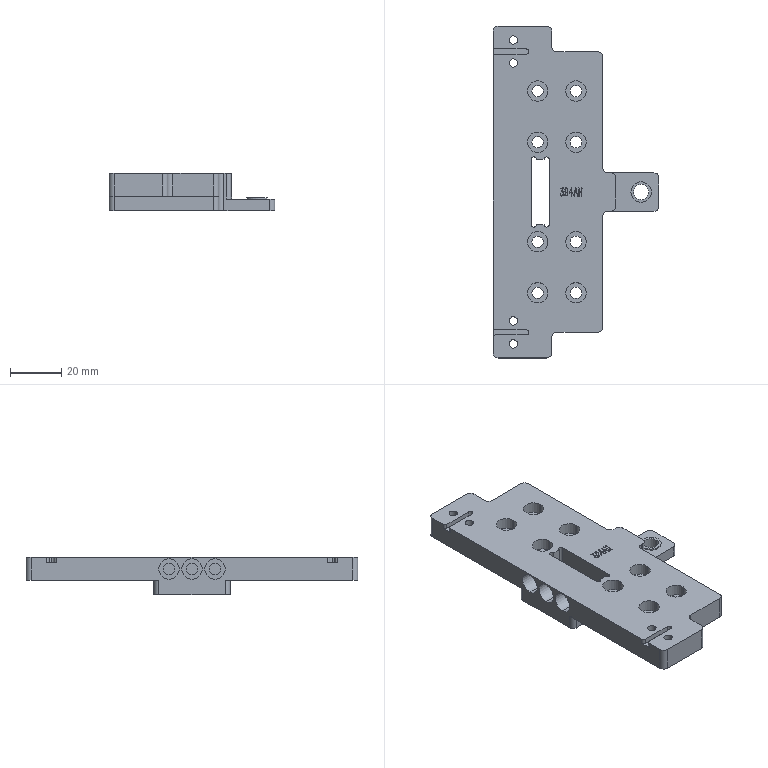NC program | NX | posted with a generic post | part box 65 x 130 x 14.5 mm
Lines 108 to 1017 of 11202:
(ADAPTIVE_MILLING , TOOL : D10)
N178 T15 M6
N180 G54
N182 G17 G0 G90 X0.062 Y-45.209 B0. C0. S9500 M3
N184 G43 Z30. H15
N186 Z-11.5
N188 G94 G1 Z-14.5 F1000.
N190 X0.341 Y-44.428 F3000.
N192 X0.597 Y-43.64
N194 G3 X0.062 Y-42.562 R1.017
N196 X-3.002 Y-41.801 R8.28
N198 X-12.869 Y-41.519 R111.643
N200 G1 X-15.119 Y-41.514
N202 X-18.994 Y-41.511
N204 X-32.619 Y-41.51
N206 X-66.869
N208 X-66.994 Y-41.509
N210 X-67.119 Y-41.508
N212 G2 X-71.4 Y-39.014 R5.714
N214 X-73.465 Y-33.574 R12.314
N216 X-73.953 Y-25.471 R57.528
N218 G1 X-73.962 Y-24.596
N220 X-73.971 Y-23.346
N222 X-73.978 Y-21.721
N224 X-73.983 Y-19.596
N226 X-73.987 Y-16.096
N228 X-73.988 Y-6.096
N230 Y34.529
N232 X-73.986 Y34.654
N234 X-73.979 Y34.779
N236 X-73.969 Y34.903
N238 G2 X-71.265 Y39.069 R5.937
N240 X-65.65 Y41.03 R13.149
N242 X-57.042 Y41.463 R69.652
N244 G1 X-55.792 Y41.472
N246 X-54.167 Y41.479
N248 X-51.917 Y41.484
N250 X-48.167 Y41.487
N252 X-36.542 Y41.488
N254 X66.958
N256 G2 X71.225 Y39.219 R5.583
N258 X73.439 Y33.711 R11.905
N260 X73.949 Y25.735 R53.792
N262 G1 X73.959 Y24.86
N264 X73.969 Y23.61
N266 X73.976 Y22.235
N268 X73.982 Y20.36
N270 X73.986 Y17.485
N272 X73.988 Y11.36
N274 Y-34.515
N276 X73.986 Y-34.639
N278 X73.98 Y-34.764
N280 X73.97 Y-34.889
N282 G2 X71.274 Y-39.06 R5.924
N284 X65.538 Y-41.044 R13.207
N286 X56.429 Y-41.467 R75.516
N288 G1 X55.054 Y-41.475
N290 X53.429 Y-41.481
N292 X50.929 Y-41.485
N294 X46.304 Y-41.488
N296 X7.804
N298 X3.804
N300 G2 X-1.419 Y-40.99 R59.156
N302 G3 X-13.656 Y-40.537 R126.191
N304 G1 X-15.531 Y-40.53
N306 X-18.031 Y-40.525
N308 X-22.031 Y-40.522
N310 X-33.531 Y-40.521
N312 X-63.906
N314 X-64.031 Y-40.519
N316 G2 X-70.336 Y-36.815 R7.665
N318 X-72.471 Y-30.468 R15.611
N320 X-72.94 Y-21.611 R73.657
N322 G1 X-72.952 Y-20.361
N324 X-72.961 Y-18.986
N326 X-72.968 Y-17.236
N328 X-72.973 Y-14.736
N330 X-72.976 Y-10.736
N332 X-72.977 Y2.389
N334 Y31.389
N336 X-72.975 Y31.639
N338 X-72.97 Y31.764
N340 X-72.964 Y31.889
N342 G2 X-69.191 Y37.896 R7.687
N344 X-62.704 Y40.003 R15.904
N346 X-53.345 Y40.449 R81.636
N348 G1 X-52.095 Y40.458
N350 X-50.345 Y40.466
N352 X-48.345 Y40.472
N354 X-45.22 Y40.475
N356 X-38.595 Y40.477
N358 X63.905 Y40.478
N360 X64.03 Y40.477
N362 X64.155 Y40.473
N364 X64.28 Y40.469
N366 X64.405 Y40.462
N368 X64.529 Y40.453
N370 G2 X70.47 Y36.567 R7.761
N372 X72.519 Y30.059 R16.204
N374 X72.954 Y20.075 R89.33
N376 G1 X72.963 Y18.575
N378 X72.969 Y16.7
N380 X72.974 Y13.95
N382 X72.977 Y9.075
N384 Y-23.675
N386 Y-31.425
N388 G2 X69.367 Y-37.779 R7.596
N390 X63.158 Y-39.93 R15.098
N392 X53.804 Y-40.444 R72.251
N394 G1 X52.679 Y-40.454
N396 X51.429 Y-40.461
N398 X49.679 Y-40.468
N400 X47.304 Y-40.473
N402 X43.304 Y-40.476
N404 X31.429 Y-40.478
N406 X6.179
N408 X5.804 Y-40.475
N410 X5.679 Y-40.474
N412 X5.304 Y-40.466
N414 X5.054 Y-40.459
N416 G2 X-3.547 Y-39.831 R349.282
N418 G3 X-18.792 Y-39.538 R283.39
N420 G1 X-22.167 Y-39.534
N422 X-28.417 Y-39.532
N424 X-60.917 Y-39.531
N426 X-61.292 Y-39.53
N428 X-61.417 Y-39.528
N430 X-61.792 Y-39.518
N432 G2 X-69.405 Y-34.81 R8.956
N434 X-71.463 Y-28.038 R17.941
N436 X-71.938 Y-17.68 R90.973
N438 G1 X-71.948 Y-16.305
N440 X-71.955 Y-14.555
N442 X-71.961 Y-12.18
N444 X-71.965 Y-8.555
N446 X-71.966 Y-0.555
N448 X-71.967 Y28.82
N450 G2 X-67.242 Y36.921 R8.928
N452 X-60.467 Y38.972 R18.132
N454 X-51.109 Y39.43 R84.153
N456 G1 X-49.859 Y39.441
N458 X-48.359 Y39.45
N460 X-46.609 Y39.457
N462 X-44.109 Y39.462
N464 X-40.109 Y39.465
N466 X-28.984 Y39.467
N468 X61.266
N470 X61.516 Y39.465
N472 X61.641 Y39.462
N474 X61.766 Y39.459
N476 X61.891 Y39.454
N478 X62.141 Y39.443
N480 G2 X69.455 Y34.676 R8.935
N482 X71.494 Y27.768 R18.331
N484 X71.945 Y16.658 R104.558
N486 G1 X71.953 Y15.033
N488 X71.959 Y13.033
N490 X71.964 Y9.908
N492 X71.966 Y4.033
N494 X71.967 Y-28.717
N496 X71.963 Y-29.092
N498 G2 X67.433 Y-36.803 R8.865
N500 X60.438 Y-38.967 R17.814
N502 X50.08 Y-39.438 R93.921
N504 G1 X48.705 Y-39.448
N506 X46.955 Y-39.455
N508 X44.58 Y-39.461
N510 X40.955 Y-39.465
N512 X33.205 Y-39.467
N514 X7.955
N516 G2 X-1.281 Y-38.989 R139.831
N518 G3 X-19.272 Y-38.552 R278.015
N520 G1 X-22.147 Y-38.547
N522 X-26.772 Y-38.544
N524 X-38.772 Y-38.542
N526 X-57.897
N528 X-58.647 Y-38.538
N530 X-59.147 Y-38.532
N532 G2 X-64.007 Y-37.537 R11.586
N534 G1 X-64.532 Y-37.477
N536 X-64.647 Y-37.451
N538 G2 X-68.548 Y-35. R7.671
N540 X-69.977 Y-32.032 R8.027
N542 X-70.926 Y-15.936 R118.648
N544 G1 X-70.936 Y-14.436
N546 X-70.943 Y-12.561
N548 X-70.949 Y-10.061
N550 X-70.953 Y-6.436
N552 X-70.955 Y0.939
N554 X-70.956 Y26.439
N556 G2 X-69.229 Y32.715 R10.337
N558 X-63.063 Y36.975 R11.915
N560 X-55.185 Y38.236 R31.194
N562 X-39.314 Y38.453 R340.669
N564 G1 X-33.189 Y38.456
N566 X58.936
N568 X59.186 Y38.455
N570 X59.436 Y38.451
N572 X59.561 Y38.448
N574 X59.811 Y38.44
N576 G2 X68.387 Y33.084 R9.805
N578 X70.469 Y25.797 R19.905
N580 X70.928 Y14.937 R106.106
N582 G1 X70.938 Y13.437
N584 X70.945 Y11.562
N586 X70.95 Y9.062
N588 X70.954 Y5.062
N590 X70.956 Y-4.313
N592 Y-26.438
N594 G2 X70.056 Y-31.334 R11.594
N596 G1 X69.977 Y-32.032
N598 X69.951 Y-32.147
N600 G2 X67.5 Y-36.048 R7.671
N602 X64.532 Y-37.477 R8.027
N604 X48.56 Y-38.425 R119.399
N606 G1 X47.06 Y-38.435
N608 X45.185 Y-38.443
N610 X42.811 Y-38.449
N612 X39.311 Y-38.453
N614 X32.561 Y-38.456
N616 X9.311
N618 G2 X-1.302 Y-37.985 R191.273
N620 G3 X-10.298 Y-37.65 R326.947
N622 G1 X-62.97
N624 X-63.03 Y-37.647
N626 X-64.023 Y-37.535
N628 X-64.336 Y-37.5
N630 X-64.647 Y-37.451
N632 G2 X-68.548 Y-35. R7.671
N634 X-69.977 Y-32.032 R8.027
N636 G1 X-70.147 Y-30.53
N638 X-70.15 Y-30.47
N640 Y-11.53
N642 G3 X-69.97 Y-0.473 R205.799
N644 G1 X-69.967 Y3.777
N646 Y23.402
N648 X-69.962 Y24.152
N650 X-69.957 Y24.652
N652 X-69.95 Y25.026
N654 X-69.943 Y25.276
N656 G2 X-64.046 Y34.868 R10.551
N658 X-56.746 Y36.921 R21.229
N660 X-46.138 Y37.409 R100.126
N662 G1 X-44.763 Y37.42
N664 X-43.138 Y37.429
N666 X-41.013 Y37.436
N668 X-38.138 Y37.441
N670 X-33.263 Y37.444
N672 X-17.013 Y37.445
N674 X-7.263
N676 X-7.138 Y37.453
N678 X-7.032 Y37.477
N680 X-5.53 Y37.647
N682 X-5.47 Y37.65
N684 X5.47
N686 G3 X17.277 Y37.47 R222.549
N688 G1 X22.277 Y37.467
N690 X55.902
N692 X56.652 Y37.462
N694 X57.152 Y37.457
N696 X57.527 Y37.451
N698 X57.776 Y37.443
N700 G2 X67.481 Y31.321 R10.587
N702 X69.447 Y23.994 R21.803
N704 X69.916 Y12.759 R111.443
N706 G1 X69.926 Y11.259
N708 X69.933 Y9.384
N710 X69.939 Y6.884
N712 X69.943 Y3.134
N714 X69.945 Y-4.866
N716 Y-9.741
N718 X69.954 Y-9.865
N720 X69.977 Y-9.968
N722 X70.147 Y-11.47
N724 X70.15 Y-11.53
N726 Y-30.47
N728 X70.147 Y-30.53
N730 X70.049 Y-31.399
N732 G3 X71.963 Y-31.902 R1.
N734 G1 X72.643 Y-30.022 Z-14.4
N736 X73.171 Y-28.556
N738 X73.212 Y-28.389
N740 X73.231 Y-28.217
N742 Y16.158
N744 G3 X72.448 Y24.837 R48.938
N746 G1 X71.853 Y28.03
N748 G3 X69.966 Y33.165 R21.419
N750 X67.55 Y36.479 R15.331
N752 X64.589 Y38.702 R15.278
N754 X59.631 Y40.225 R13.173
N756 X53.401 Y40.489 R88.661
N758 G1 X8.712 Y40.829
N760 X8.525 Y40.808
N762 X8.342 Y40.761
N764 X6.542 Y40.062
N766 X5.834 Y39.793 Z-14.438
N768 X5.135 Y39.502 Z-14.476
N770 X4.945 Y39.353 Z-14.488
N772 X4.791 Y39.167 Z-14.5
N774 G3 X5.53 Y37.647 R1.002
N776 G2 X8.218 Y37.109 R8.94
N778 G3 X14.307 Y36.551 R31.104
N780 X27.432 Y36.478 R710.533
N782 G1 X47.432
N784 X52.932
N786 X54.057 Y36.471
N788 X55.057 Y36.463
N790 X55.432 Y36.457
N792 G2 X61.375 Y35.23 R13.199
N794 X66.904 Y28.858 R11.902
N796 X68.543 Y21.185 R26.67
N798 X68.914 Y9.445 R144.37
N800 G1 X68.922 Y7.445
N802 X68.928 Y4.82
N804 X68.932 Y0.945
N806 X68.934 Y-6.68
N808 X68.937 Y-7.18
N810 X68.938 Y-7.305
N812 G3 X69.41 Y-8.347 R2.177
N814 G1 X69.462 Y-8.454
N816 X69.951 Y-9.853
N818 X69.977 Y-9.968
N820 G3 X71.777 Y-10.311 R1.001
N822 X71.964 Y-9.624 Z-14.464 R1.251
N824 G1 X72.06 Y-8.351 Z-14.4
N826 X72.227 Y-6.071
N828 Y12.679
N830 G3 X71.467 Y22.621 R65.951
N832 G1 X70.865 Y26.447
N834 G3 X69.412 Y31.071 R19.913
N836 X65.701 Y35.996 R14.244
N838 X59.036 Y39.105 R12.236
N840 X54.69 Y39.47 R37.522
N842 G1 X10.919 Y40.427
N844 X10.704 Y40.404
N846 X10.496 Y40.343
N848 X8.72 Y39.566
N850 X8.114 Y39.306 Z-14.433
N852 X7.517 Y39.024 Z-14.466
N854 G3 X7.115 Y38.492 Z-14.5 R1.039
N856 X7.737 Y37.245 R1.005
N858 G2 X9.436 Y36.523 R12.4
N860 G3 X14.6 Y35.68 R18.818
N862 X26.722 Y35.493 R258.293
N864 G1 X30.722 Y35.49
N866 X42.597 Y35.488
N868 X49.847
N870 X50.347 Y35.486
N872 X53.222 Y35.465
N874 X53.597 Y35.461
N876 G2 X59.47 Y34.452 R15.167
N878 X65.585 Y28.143 R11.91
N880 X67.465 Y20.275 R25.475
N882 X67.904 Y7.162 R147.503
N884 G3 X67.964 Y-5.713 R786.636
N886 X68.622 Y-7.093 R1.753
N888 G1 X69.087 Y-7.833
N890 G3 X70.475 Y-8.142 R1.004
N892 X70.949 Y-7.235 Z-14.447 R1.113
N894 G1 X71.06 Y-6.308 Z-14.4
N896 X71.337 Y-3.936
N898 Y11.064
N900 G3 X70.515 Y20.996 R60.929
N902 G1 X69.954 Y24.279
N904 G3 X68.246 Y29.569 R23.438
N906 X66.391 Y32.578 R17.281
N908 G1 X65.44 Y33.814
N910 X64.452 Y35.023
N912 G3 X63.502 Y35.812 R4.158
N914 G1 X62.509 Y36.405
N916 X61.491 Y36.954
N918 G3 X58.259 Y37.964 R12.606
N920 X55.294 Y38.29 R21.54
N922 X44.055 Y38.612 R487.31
N924 G1 X12.656 Y39.094
N926 X10.323 Y38.822
N928 X9.663 Y38.748 Z-14.433
N930 X9.007 Y38.649 Z-14.466
N932 G3 X8.472 Y38.264 Z-14.5 R1.04
N934 X8.759 Y36.844 R1.004
N936 X13.595 Y35.011 R9.961
N938 X22.951 Y34.534 R74.786
N940 G1 X24.076 Y34.524
N942 X25.576 Y34.515
N944 X27.451 Y34.508
N946 X30.076 Y34.503
N948 X34.451 Y34.5
N950 X46.826 Y34.499
N952 G2 X54.323 Y34.341 R110.325
N954 X64.232 Y27.506 R11.875
N956 X66.331 Y19.826 R23.732
N958 X66.868 Y8.595 R103.424
N960 G3 X66.975 Y-4.279 R570.276
N962 X67.296 Y-5.729 R3.252
N964 G1 X67.371 Y-5.829
N966 X67.451 Y-5.913
N968 X67.5 Y-5.952
N970 X68.296 Y-6.748
N972 G3 X69.493 Y-6.912 R1.007
N974 X70.02 Y-6.026 Z-14.446 R1.11
N976 G1 X70.175 Y-5.114 Z-14.4
N978 X70.531 Y-3.018
N980 X70.546 Y-2.85
N982 X70.552 Y2.304
N984 X70.532 Y7.459
N986 G3 X69.662 Y18.337 R88.999
N988 G1 X68.944 Y23.283
N990 G3 X66.499 Y29.632 R17.756
N992 X63.652 Y33.467 R33.142
N994 X61.538 Y35.095 R8.254
N996 X57.53 Y36.767 R19.734
N998 X54.779 Y37.262 R17.832
N1000 G1 X53.381 Y37.384
N1002 X51.98 Y37.452
N1004 X13.805 Y38.372
N1006 X13.638 Y38.362
N1008 X11.517 Y38.056
N1010 X10.867 Y37.968 Z-14.433
N1012 X10.221 Y37.854 Z-14.466
N1014 G3 X9.688 Y37.442 Z-14.5 R1.039
N1016 X9.907 Y36.122 R1.005
N1018 X13.061 Y34.458 R6.193
N1020 X20.002 Y33.656 R34.038
N1022 X40.876 Y33.51 R729.268
N1024 G2 X52.374 Y33.382 R246.99
N1026 X60.504 Y30.01 R12.436
N1028 X64.46 Y22.881 R15.607
N1030 X65.685 Y13.857 R42.285
N1032 X65.927 Y-1.765 R504.611
N1034 G3 X66.356 Y-4.972 R10.178
N1036 X66.728 Y-5.451 R1.974
N1038 G1 X67.407 Y-5.878
N1040 X67.5 Y-5.952
N1042 G3 X68.593 Y-6.053 R1.01
N1044 X69.141 Y-5.185 Z-14.447 R1.112
N1046 G1 X69.324 Y-4.273 Z-14.4
N1048 X69.745 Y-2.154
N1050 X69.749 Y0.811
N1052 X69.736 Y3.777
N1054 G3 X69.239 Y11.04 R76.64
N1056 G1 X68.071 Y20.972
N1058 G3 X66.059 Y27.351 R18.53
N1060 X63.548 Y31.057 R19.959
N1062 G1 X62.05 Y32.782
N1064 G3 X59.881 Y34.33 R7.933
N1066 X55.808 Y35.836 R19.367
N1068 G1 X54.894 Y36.009
N1070 X53.972 Y36.128
N1072 G3 X46.502 Y36.661 R140.558
N1074 G1 X14.056 Y38.032
N1076 X11.925 Y37.669
N1078 X11.278 Y37.563 Z-14.433
N1080 X10.636 Y37.432 Z-14.466
N1082 G3 X10.114 Y37.004 Z-14.5 R1.038
N1084 X10.265 Y35.783 R1.007
N1086 X14.066 Y33.558 R6.919
N1088 X21.375 Y32.684 R35.467
N1090 X41.373 Y32.519 R649.43
N1092 G2 X51.245 Y32.361 R184.013
N1094 X59.453 Y28.85 R12.682
N1096 X63.438 Y21.594 R15.962
N1098 X64.678 Y12.194 R43.946
N1100 X64.939 Y-0.928 R757.799
N1102 G3 X65.511 Y-4.488 R10.583
N1104 X66.153 Y-5.09 R1.269
N1106 G1 X66.788 Y-5.489
N1108 G3 X67.857 Y-5.486 R1.011
N1110 X68.336 Y-4.695 Z-14.452 R1.141
N1112 G1 X68.584 Y-3.679 Z-14.4
N1114 X69.013 Y-1.919
N1116 X69.035 Y-1.756
N1118 X69.038 Y-1.592
N1120 X67.34 Y17.081
N1122 G3 X64.735 Y26.656 R28.478
N1124 G1 X64.115 Y27.973
N1126 X63.477 Y29.281
N1128 G3 X62.196 Y30.876 R6.306
N1130 X60.187 Y32.344 R13.52
N1132 G1 X58.031 Y33.605
N1134 G3 X54.422 Y34.899 R13.803
N1136 X51.465 Y35.296 R19.423
N1138 G1 X14.945 Y37.25
N1140 X14.691 Y37.231
N1142 X12.77 Y36.837
N1144 X12.117 Y36.708 Z-14.433
N1146 X11.469 Y36.556 Z-14.467
N1148 G3 X10.969 Y36.132 Z-14.5 R1.04
N1150 X11.048 Y35. R1.01
N1152 X13.483 Y33.144 R4.764
N1154 X19.71 Y31.891 R21.941
N1156 X33.328 Y31.544 R186.85
N1158 G2 X48.951 Y31.42 R720.332
N1160 X55.686 Y29.76 R15.123
N1162 X61.612 Y22.737 R13.595
N1164 X63.436 Y14.211 R30.177
N1166 X63.886 Y1.471 R195.494
N1168 G3 X64.399 Y-3.364 R20.481
N1170 X65.108 Y-4.659 R2.532
N1172 X66.031 Y-5.033 R5.554
N1174 X67.056 Y-4.808 R1.011
N1176 X67.355 Y-3.944 Z-14.453 R1.045
N1178 G1 X67.303 Y-2.893 Z-14.4
N1180 X67.196 Y-0.686
N1182 X67.199 Y3.062
N1184 X67.184 Y6.811
N1186 G3 X66.435 Y15.505 R66.209
N1188 G1 X65.834 Y19.331
N1190 G3 X63.076 Y26.434 R20.586
N1192 X61.18 Y29.178 R29.442
N1194 X57.298 Y32.365 R13.139
N1196 X52.012 Y34.101 R15.564
N1198 X48.287 Y34.439 R41.618
N1200 G1 X15.538 Y35.865
N1202 X13.33 Y36.102
N1204 X12.683 Y36.177 Z-14.433
N1206 X12.034 Y36.226 Z-14.465
N1208 G3 X11.409 Y35.949 Z-14.5 R1.038
N1210 X11.255 Y34.696 R1.007
N1212 X14.048 Y32.32 R5.139
N1214 X20.255 Y30.972 R21.659
N1216 X32.619 Y30.566 R150.127
N1218 G2 X47.618 Y30.419 R690.232
N1220 X54.482 Y28.755 R15.699
N1222 X60.481 Y21.791 R13.69
N1224 X62.393 Y13.16 R29.577
N1226 X62.87 Y2.422 R176.912
N1228 G3 X63.426 Y-2.661 R23.392
N1230 X64.234 Y-4.329 R3.629
N1232 X65.355 Y-4.797 R4.211
N1234 X66.415 Y-4.536 R1.01
N1236 X66.679 Y-3.704 Z-14.455 R1.051
N1238 G1 X66.626 Y-2.607 Z-14.4
N1240 X66.508 Y0.031
N1242 X66.442 Y2.67
N1244 G3 X65.978 Y8.887 R64.502
N1246 G1 X65.402 Y13.54
N1248 X64.804 Y18.19
N1250 G3 X62.487 Y24.6 R19.116
N1252 G1 X61.696 Y25.982
N1254 X60.89 Y27.356
N1256 G3 X59.53 Y28.885 R7.197
N1258 X56.138 Y31.324 R27.641
N1260 X52.511 Y32.731 R13.66
N1262 X49.438 Y33.215 R20.528
N1264 G1 X46.951 Y33.435
N1266 X44.46 Y33.608
N1268 X15.951 Y35.229
N1270 X13.737 Y35.466
N1272 X13.087 Y35.541 Z-14.433
N1274 X12.435 Y35.591 Z-14.466
N1276 G3 X11.814 Y35.32 Z-14.5 R1.038
N1278 X11.654 Y34.061 R1.007
N1280 X14.448 Y31.54 R5.23
N1282 X20.873 Y30.041 R21.18
N1284 X32.11 Y29.593 R127.475
N1286 G2 X46.483 Y29.411 R554.904
N1288 X53.452 Y27.662 R15.796
N1290 X59.479 Y20.559 R13.94
N1292 X61.341 Y12.295 R29.893
N1294 X61.894 Y2.187 R220.15
N1296 G3 X62.707 Y-2.855 R18.132
N1298 X63.641 Y-4.306 R3.138
N1300 X64.647 Y-4.549 R2.756
N1302 X65.59 Y-4.268 R1.014
N1304 X65.867 Y-3.371 Z-14.452 R1.133
N1306 G1 X65.85 Y-2.341 Z-14.4
N1308 X65.812 Y-0.202
N1310 X64.087 Y15.327
N1312 G3 X61.957 Y22.458 R21.485
N1314 G1 X60.835 Y24.684
N1316 G3 X58.138 Y28.033 R12.939
N1318 X54.034 Y30.807 R15.608
N1320 X50.469 Y31.857 R14.551
N1322 X45.526 Y32.513 R45.278
N1324 G1 X16.282 Y34.712
N1326 X14.136 Y34.817
N1328 X13.464 Y34.855 Z-14.434
N1330 X12.791 Y34.87 Z-14.467
N1332 G3 X12.211 Y34.595 Z-14.5 R1.041
N1334 X11.962 Y33.546 R1.01
N1336 X13.819 Y31.285 R3.896
N1338 X19.1 Y29.449 R14.901
N1340 X29.435 Y28.664 R69.044
N1342 G2 X45.183 Y28.418 R972.185
N1344 X52.059 Y26.78 R16.577
N1346 X58.367 Y19.61 R13.894
N1348 X60.368 Y10.615 R30.508
N1350 G1 X60.402 Y10.242
N1352 X60.434 Y9.868
N1354 X60.482 Y9.245
N1356 X60.518 Y8.746
N1358 X60.56 Y8.123
N1360 X60.598 Y7.499
N1362 X60.654 Y6.501
N1364 X60.734 Y5.003
N1366 X60.779 Y4.254
N1368 X60.834 Y3.381
N1370 X60.876 Y2.757
N1372 X60.916 Y2.259
N1374 X60.948 Y1.885
N1376 X60.983 Y1.512
N1378 G3 X62.053 Y-3.092 R13.998
N1380 X63.077 Y-4.314 R2.455
N1382 X64.047 Y-4.468 R6.205
N1384 X64.954 Y-4.08 R1.014
N1386 X65.162 Y-3.297 Z-14.459 R1.193
N1388 G1 X65.184 Y-2.125 Z-14.4
N1390 X65.207 Y-1.123
N1392 X65.211 Y-0.121
N1394 X64.443 Y5.951
N1396 G3 X63.256 Y12.842 R116.68
N1398 G1 X62.807 Y15.046
N1400 X62.342 Y17.248
N1402 G3 X59.441 Y23.963 R21.185
N1404 X57.732 Y26.421 R28.578
N1406 X55.48 Y28.356 R9.402
N1408 G1 X54.835 Y28.733
N1410 X54.171 Y29.076
N1412 G3 X51.319 Y30.325 R31.325
N1414 X48.299 Y31.038 R12.343
N1416 G1 X18.085 Y34.083
N1418 X16.426 Y34.242
N1420 X14.339 Y34.344
N1422 X13.652 Y34.381 Z-14.434
N1424 X12.964 Y34.399 Z-14.469
N1426 G3 X12.403 Y34.149 Z-14.5 R1.045
N1428 X12.127 Y33.074 R1.01
N1430 X14.153 Y30.485 R4.278
N1432 X19.653 Y28.525 R15.341
N1434 X29.609 Y27.701 R65.74
N1436 G2 X43.981 Y27.421 R927.051
N1438 X50.864 Y25.8 R17.016
N1440 X57.345 Y18.461 R14.093
N1442 X59.015 Y12.324 R28.906
N1444 X59.977 Y10.032 R8.084
N1446 G1 X60.147 Y8.53
N1448 X60.15 Y8.47
N1450 G3 X60.204 Y1.347 R138.36
N1452 X61.449 Y-3.325 R11.08
N1454 X62.643 Y-4.344 R1.819
N1456 G1 X62.688 Y-4.35
N1458 X62.97
N1460 X63.03 Y-4.353
N1462 X63.402 Y-4.395
N1464 G3 X64.546 Y-2.891 R1.102
N1466 G1 X62.27 Y2.756
N1468 G3 X60.15 Y2.345 R1.1
N1470 X60.2 Y-1.402 R46.797
N1472 X61.529 Y-4.156 R4.331
N1474 X62.697 Y-4.35 R1.957
N1476 X63.646 Y-2.694 R1.102
N1478 G1 X62.199 Y-0.224
N1480 G3 X60.15 Y-0.78 R1.101
N1482 X60.268 Y-2.893 R8.097
N1484 X61.257 Y-4.27 R2.011
N1486 X62.086 Y-4.35 R2.566
N1488 X62.96 Y-2.583 R1.101
N1490 G1 X62.124 Y-1.487
N1492 G3 X60.15 Y-2.155 R1.101
N1494 X60.426 Y-3.854 R3.024
N1496 X61.638 Y-4.35 R1.258
N1498 X62.369 Y-2.428 R1.101
N1500 G1 X61.837 Y-1.975
N1502 G3 X60.15 Y-2.905 R1.102
N1504 X60.681 Y-4.208 R1.297
N1506 X61.338 Y-4.35 R1.554
N1508 X62.171 Y-3.902 R1.014
N1510 G1 X62.395 Y-3.565
N1512 X63.499 Y-1.897 Z-14.4
N1514 X63.683 Y-1.62
N1516 X63.909 Y-1.376
N1518 G2 X64.519 Y-1.168 R1.041
N1520 G1 X65.292 Y-1.166
N1522 X66.065 Y-1.183
N1524 G2 X67.903 Y-2.052 R3.052
N1526 G1 X69.38 Y-3.521
N1528 X70.839 Y-5.006
N1530 G2 X72.193 Y-7.296 R7.593
N1532 X73.164 Y-11.513 R13.709
N1534 G1 X73.365 Y-14.789
N1536 X73.551 Y-18.066
N1538 G2 X73.312 Y-28.974 R85.567
N1540 G1 X73.12 Y-31.265
N1542 X72.902 Y-33.554
N1544 G2 X71.136 Y-37.052 R6.303
N1546 G1 X70.499 Y-37.687
N1548 X69.827 Y-38.284
N1550 G2 X68.223 Y-39.282 R8.641
N1552 G1 X67.503 Y-39.631
N1554 X66.771 Y-39.955
N1556 G2 X65.81 Y-39.719 R1.016
N1558 G1 X64.311 Y-38.394 Z-14.5
N1560 X63.624 Y-37.802
N1562 G3 X63.03 Y-37.647 R1.045
N1564 G1 X62.97 Y-37.65
N1566 X-10.405
N1568 G3 X-11.238 Y-38.098 R1.014
N1570 G1 X-11.439 Y-38.4
N1572 X-12.543 Y-40.068 Z-14.4
N1574 X-12.855 Y-40.513
N1576 G2 X-13.587 Y-40.832 R1.026
N1578 G1 X-61.712
N1580 G2 X-66.912 Y-39.854 R13.998
N1582 X-70.058 Y-37.918 R10.907
N1584 X-72.636 Y-33.851 R8.768
N1586 G1 X-72.82 Y-33.038
N1588 X-72.95 Y-32.214
N1590 G2 X-73.167 Y-29.235 R25.387
N1592 G1 X-73.329 Y-14.652
N1594 G2 X-72.904 Y-13.824 R1.015
N1596 G1 X-72.668 Y-13.657
N1598 X-71.033 Y-12.506 Z-14.5
N1600 X-70.435 Y-12.068
N1602 G3 X-70.147 Y-11.47 R1.039
N1604 G2 X-69.607 Y-8.782 R8.856
N1606 G3 X-69.047 Y-2.568 R31.948
N1608 X-68.978 Y11.557 R744.469
N1610 G2 X-68.91 Y24.181 R411.179
N1612 X-62.501 Y33.891 R11.074
N1614 X-54.685 Y35.95 R23.171
N1616 X-42.449 Y36.41 R127.939
N1618 G1 X-40.699 Y36.419
N1620 X-38.574 Y36.426
N1622 X-35.574 Y36.43
N1624 X-30.574 Y36.433
N1626 X-13.699 Y36.435
N1628 X-10.324
N1630 G3 X-8.653 Y36.91 R2.161
N1632 G1 X-8.546 Y36.962
N1634 X-7.147 Y37.451
N1636 X-7.032 Y37.477
N1638 G3 X-6.689 Y39.277 R1.001
N1640 X-7.376 Y39.464 Z-14.464 R1.251
N1642 G1 X-8.649 Y39.56 Z-14.4
N1644 X-10.929 Y39.727
N1646 X-46.554
N1648 G3 X-55.244 Y39.008 R53.484
N1650 G1 X-56.989 Y38.718
N1652 X-58.725 Y38.38
N1654 G3 X-63.667 Y36.805 R29.466
N1656 X-67.886 Y33.913 R13.629
N1658 X-69.864 Y31.426 R17.509
N1660 X-71.218 Y28.235 R10.347
N1662 X-71.846 Y23.942 R21.013
N1664 G1 X-72.927 Y-6.081
N1666 X-72.906 Y-6.304
N1668 X-72.843 Y-6.519
N1670 X-72.066 Y-8.285
N1672 X-71.805 Y-8.89 Z-14.433
N1674 X-71.522 Y-9.485 Z-14.466
N1676 G3 X-70.987 Y-9.887 Z-14.5 R1.039
N1678 X-69.745 Y-9.263 R1.005
N1680 G2 X-69.023 Y-7.565 R12.421
N1682 G3 X-68.188 Y-2.525 R18.43
N1684 X-67.99 Y12.847 R318.555
N1686 G2 X-67.899 Y22.72 R226.254
N1688 X-61.1 Y32.875 R11.554
N1690 X-53.276 Y34.911 R23.885
N1692 X-40.916 Y35.396 R125.265
N1694 G1 X-39.291 Y35.405
N1696 X-37.166 Y35.413
N1698 X-34.291 Y35.419
N1700 X-30.041 Y35.422
N1702 X-20.041 Y35.424
N1704 X-13.416
N1706 G3 X-10.674 Y35.549 R17.041
N1708 X-9.907 Y36.122 R2.415
N1710 G1 X-9.167 Y36.587
N1712 G3 X-8.858 Y37.975 R1.004
N1714 X-9.765 Y38.449 Z-14.447 R1.113
N1716 G1 X-10.692 Y38.56 Z-14.4
N1718 X-13.064 Y38.837
N1720 X-39.933 Y38.736
N1722 G3 X-51.156 Y38.166 R121.404
N1724 G1 X-54.528 Y37.822
N1726 G3 X-59.734 Y36.677 R30.494
N1728 G1 X-60.828 Y36.334
N1730 X-61.905 Y35.944
N1732 G3 X-64.843 Y34.25 R14.3
N1734 X-69.949 Y27.649 R14.021
N1736 X-70.463 Y25.599 R13.576
N1738 X-70.876 Y21.889 R23.02
N1740 G1 X-71.594 Y-4.344
N1742 X-71.47 Y-5.513
N1744 X-71.322 Y-6.678
N1746 X-71.248 Y-7.338 Z-14.433
N1748 X-71.149 Y-7.994 Z-14.466
N1750 G3 X-70.763 Y-8.529 Z-14.5 R1.04
N1752 X-69.344 Y-8.241 R1.004
N1754 X-67.511 Y-3.405 R9.953
N1756 X-67.036 Y5.701 R73.214
N1758 G2 X-66.927 Y20.7 R888.784
N1760 X-64.833 Y27.666 R12.926
N1762 X-58.056 Y32.56 R13.512
N1764 X-49.344 Y34.107 R32.844
N1766 X-35.6 Y34.401 R231.971
N1768 G1 X-32.975 Y34.407
N1770 X-28.975 Y34.411
N1772 X-20.85 Y34.413
N1774 X-16.35
N1776 X-15.225 Y34.42
N1778 X-14.225 Y34.428
N1780 G3 X-11.495 Y34.676 R11.003
N1782 X-11.048 Y35. R2.38
N1784 G1 X-10.252 Y35.796
N1786 G3 X-10.088 Y36.993 R1.007
N1788 X-10.974 Y37.52 Z-14.446 R1.11
N1790 G1 X-11.886 Y37.675 Z-14.4
N1792 X-13.982 Y38.031
N1794 X-14.15 Y38.046
N1796 X-37.275
N1798 G3 X-50.955 Y37.073 R97.54
N1800 G1 X-55.486 Y36.414
N1802 G3 X-62.1 Y34.267 R24.866
N1804 X-65.185 Y32.01 R12.628
N1806 G1 X-65.98 Y31.217
N1808 X-66.742 Y30.393
N1810 G3 X-68.705 Y26.956 R10.644
N1812 X-69.739 Y22.106 R17.615
N1814 X-70.072 Y17.124 R96.984
N1816 G1 X-70.871 Y-3.287
N1818 X-70.557 Y-5.483
N1820 X-70.468 Y-6.133 Z-14.433
N1822 X-70.354 Y-6.78 Z-14.466
N1824 G3 X-69.942 Y-7.312 Z-14.5 R1.039
N1826 X-68.622 Y-7.093 R1.005
N1828 X-66.958 Y-3.939 R6.194
N1830 X-66.146 Y3.252 R34.939
N1832 X-65.963 Y18.251 R890.051
N1834 G2 X-64.909 Y24.373 R16.752
N1836 X-58.438 Y30.847 R12.446
N1838 X-50.227 Y32.89 R25.971
N1840 X-37.866 Y33.371 R132.287
N1842 G1 X-36.366 Y33.38
N1844 X-34.367 Y33.389
N1846 X-31.867 Y33.395
N1848 X-28.117 Y33.399
N1850 X-21.367 Y33.402
N1852 X-19.367
N1854 X-18.867 Y33.405
N1856 G3 X-13.123 Y33.582 R54.793
N1858 X-11.626 Y34.136 R2.578
N1860 G1 X-11.549 Y34.228
N1862 X-11.122 Y34.907
N1864 X-11.048 Y35.
N1866 G3 X-10.947 Y36.093 R1.01
N1868 X-11.815 Y36.641 Z-14.447 R1.112
N1870 G1 X-12.727 Y36.824 Z-14.4
N1872 X-14.846 Y37.245
N1874 X-32.445 Y37.25
N1876 G3 X-47.387 Y36.32 R121.472
N1878 G1 X-50.55 Y35.929
N1880 X-53.709 Y35.516
N1882 G3 X-60.087 Y33.438 R22.281
N1884 X-65.059 Y29.791 R15.678
N1886 X-67.393 Y26.18 R11.285
N1888 X-68.63 Y21.761 R19.653
N1890 G1 X-68.784 Y20.651
N1892 X-68.895 Y19.537
N1894 X-70.533 Y-2.838
N1896 X-70.52 Y-3.083
N1898 X-70.172 Y-5.074
N1900 X-70.064 Y-5.722 Z-14.433
N1902 X-69.931 Y-6.365 Z-14.466
N1904 G3 X-69.504 Y-6.885 Z-14.5 R1.039
N1906 X-68.283 Y-6.735 R1.007
N1908 X-66.06 Y-2.933 R6.911
N1910 X-65.19 Y4.251 R34.83
N1912 X-64.953 Y17.373 R897.345
N1914 G2 X-63.591 Y23.805 R15.735
N1916 X-56.814 Y29.988 R13.051
N1918 X-48.567 Y31.901 R27.686
N1920 X-35.08 Y32.367 R153.586
N1922 G1 X-33.205 Y32.375
N1924 X-30.955 Y32.382
N1926 X-27.83 Y32.387
N1928 X-22.455 Y32.39
N1930 X-21.955 Y32.392
N1932 X-20.205 Y32.404
N1934 X-19.705 Y32.406
N1936 G3 X-13.841 Y32.65 R41.883
N1938 X-12.206 Y33.217 R3.471
N1940 X-11.511 Y34.288 R9.301
N1942 X-11.516 Y35.359 R1.011
N1944 X-12.313 Y35.837 Z-14.452 R1.139
N1946 G1 X-13.326 Y36.076 Z-14.4
N1948 X-15.289 Y36.532
N1950 X-20.815 Y36.508
N1952 X-26.341 Y36.452
N1954 G3 X-41.611 Y35.59 R200.773
N1956 G1 X-46.323 Y35.147
N1958 X-51.034 Y34.681
N1960 G3 X-55.181 Y33.737 R22.411
N1962 X-58.692 Y32.441 R35.301
N1964 X-61.392 Y30.89 R16.807
N1966 X-64.605 Y27.973 R15.506
N1968 X-66.598 Y24.553 R10.754
N1970 X-67.753 Y19.337 R22.668
N1972 G1 X-69.75 Y-2.055
N1974 X-69.733 Y-2.352
N1976 X-69.341 Y-4.233
N1978 X-69.21 Y-4.886 Z-14.433
N1980 X-69.055 Y-5.534 Z-14.467
N1982 G3 X-68.63 Y-6.033 Z-14.5 R1.04
N1984 X-67.5 Y-5.952 R1.01
N1986 X-65.645 Y-3.515 R4.777
N1988 X-64.403 Y2.587 R21.662
N1990 X-64.022 Y14.078 R181.034